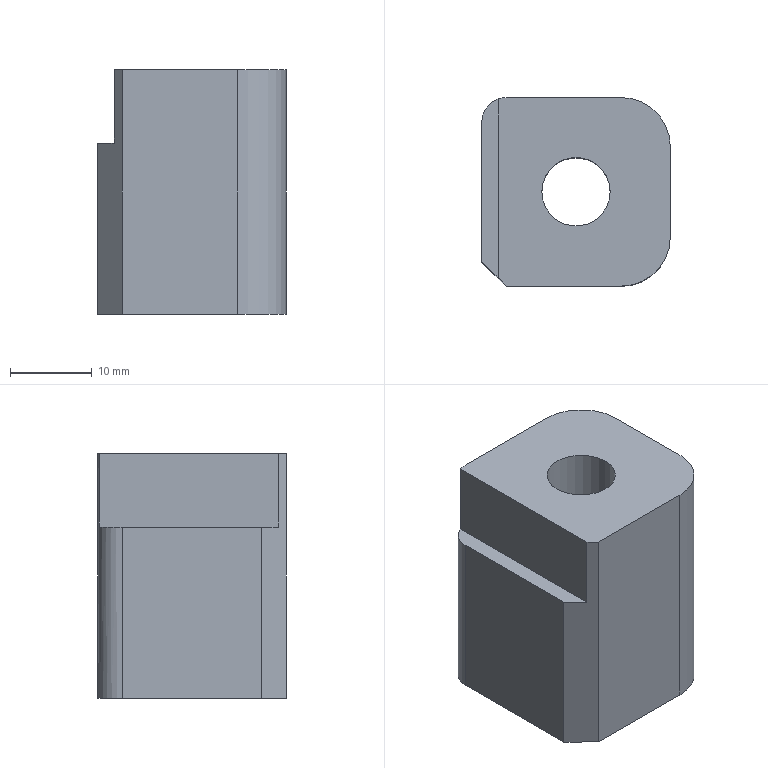Part | STEP file | 1 solid | 13 faces | box 23.1 x 23.1 x 30 mm | volume 13334 mm3 | plane 9 | cylinder 4 | commonest cylinder face diameters 12 x2 6 x1 8.38 x1
STEP:
#1=CARTESIAN_POINT('',(-203.45,11.55,-32.));
#2=VERTEX_POINT('',#1);
#3=CARTESIAN_POINT('',(-217.55,11.55,-32.));
#4=VERTEX_POINT('',#3);
#5=CARTESIAN_POINT('',(-209.,11.55,-32.));
#6=DIRECTION('',(-1.,0.,0.));
#7=VECTOR('',#6,1.);
#8=LINE('',#5,#7);
#9=EDGE_CURVE('',#2,#4,#8,.T.);
#10=ORIENTED_EDGE('',*,*,#9,.T.);
#11=CARTESIAN_POINT('',(-217.55,11.55,-2.));
#12=VERTEX_POINT('',#11);
#13=CARTESIAN_POINT('',(-217.55,11.55,-30.));
#14=DIRECTION('',(0.,0.,1.));
#15=VECTOR('',#14,1.);
#16=LINE('',#13,#15);
#17=EDGE_CURVE('',#4,#12,#16,.T.);
#18=ORIENTED_EDGE('',*,*,#17,.T.);
#19=CARTESIAN_POINT('',(-203.45,11.55,-2.));
#20=VERTEX_POINT('',#19);
#21=CARTESIAN_POINT('',(-209.,11.55,-2.));
#22=DIRECTION('',(1.,0.,0.));
#23=VECTOR('',#22,1.);
#24=LINE('',#21,#23);
#25=EDGE_CURVE('',#12,#20,#24,.T.);
#26=ORIENTED_EDGE('',*,*,#25,.T.);
#27=CARTESIAN_POINT('',(-203.45,11.55,-30.));
#28=DIRECTION('',(0.,0.,-1.));
#29=VECTOR('',#28,1.);
#30=LINE('',#27,#29);
#31=EDGE_CURVE('',#20,#2,#30,.T.);
#32=ORIENTED_EDGE('',*,*,#31,.T.);
#33=EDGE_LOOP('',(#10,#18,#26,#32));
#34=FACE_OUTER_BOUND('',#33,.T.);
#35=CARTESIAN_POINT('',(-209.,11.55,-30.));
#36=DIRECTION('',(0.,1.,0.));
#37=DIRECTION('',(0.,0.,-1.));
#38=AXIS2_PLACEMENT_3D('',#35,#36,#37);
#39=PLANE('',#38);
#40=ADVANCED_FACE('',(#34),#39,.T.);
#41=CARTESIAN_POINT('',(-197.45,5.55,-2.));
#42=VERTEX_POINT('',#41);
#43=CARTESIAN_POINT('',(-197.45,-5.55,-2.));
#44=VERTEX_POINT('',#43);
#45=CARTESIAN_POINT('',(-197.45,0.,-2.));
#46=DIRECTION('',(0.,-1.,0.));
#47=VECTOR('',#46,1.);
#48=LINE('',#45,#47);
#49=EDGE_CURVE('',#42,#44,#48,.T.);
#50=ORIENTED_EDGE('',*,*,#49,.T.);
#51=CARTESIAN_POINT('',(-197.45,-5.55,-32.));
#52=VERTEX_POINT('',#51);
#53=CARTESIAN_POINT('',(-197.45,-5.55,-30.));
#54=DIRECTION('',(0.,0.,-1.));
#55=VECTOR('',#54,1.);
#56=LINE('',#53,#55);
#57=EDGE_CURVE('',#44,#52,#56,.T.);
#58=ORIENTED_EDGE('',*,*,#57,.T.);
#59=CARTESIAN_POINT('',(-197.45,5.55,-32.));
#60=VERTEX_POINT('',#59);
#61=CARTESIAN_POINT('',(-197.45,0.,-32.));
#62=DIRECTION('',(0.,1.,0.));
#63=VECTOR('',#62,1.);
#64=LINE('',#61,#63);
#65=EDGE_CURVE('',#52,#60,#64,.T.);
#66=ORIENTED_EDGE('',*,*,#65,.T.);
#67=CARTESIAN_POINT('',(-197.45,5.55,-30.));
#68=DIRECTION('',(0.,0.,1.));
#69=VECTOR('',#68,1.);
#70=LINE('',#67,#69);
#71=EDGE_CURVE('',#60,#42,#70,.T.);
#72=ORIENTED_EDGE('',*,*,#71,.T.);
#73=EDGE_LOOP('',(#50,#58,#66,#72));
#74=FACE_OUTER_BOUND('',#73,.T.);
#75=CARTESIAN_POINT('',(-197.45,0.,-30.));
#76=DIRECTION('',(1.,0.,0.));
#77=DIRECTION('',(0.,0.,1.));
#78=AXIS2_PLACEMENT_3D('',#75,#76,#77);
#79=PLANE('',#78);
#80=ADVANCED_FACE('',(#74),#79,.T.);
#81=CARTESIAN_POINT('',(-203.45,-11.55,-2.));
#82=VERTEX_POINT('',#81);
#83=CARTESIAN_POINT('',(-217.55,-11.55,-2.));
#84=VERTEX_POINT('',#83);
#85=CARTESIAN_POINT('',(-209.,-11.55,-2.));
#86=DIRECTION('',(-1.,0.,0.));
#87=VECTOR('',#86,1.);
#88=LINE('',#85,#87);
#89=EDGE_CURVE('',#82,#84,#88,.T.);
#90=ORIENTED_EDGE('',*,*,#89,.T.);
#91=CARTESIAN_POINT('',(-217.55,-11.55,-32.));
#92=VERTEX_POINT('',#91);
#93=CARTESIAN_POINT('',(-217.55,-11.55,-30.));
#94=DIRECTION('',(0.,0.,-1.));
#95=VECTOR('',#94,1.);
#96=LINE('',#93,#95);
#97=EDGE_CURVE('',#84,#92,#96,.T.);
#98=ORIENTED_EDGE('',*,*,#97,.T.);
#99=CARTESIAN_POINT('',(-203.45,-11.55,-32.));
#100=VERTEX_POINT('',#99);
#101=CARTESIAN_POINT('',(-209.,-11.55,-32.));
#102=DIRECTION('',(1.,0.,0.));
#103=VECTOR('',#102,1.);
#104=LINE('',#101,#103);
#105=EDGE_CURVE('',#92,#100,#104,.T.);
#106=ORIENTED_EDGE('',*,*,#105,.T.);
#107=CARTESIAN_POINT('',(-203.45,-11.55,-30.));
#108=DIRECTION('',(0.,0.,1.));
#109=VECTOR('',#108,1.);
#110=LINE('',#107,#109);
#111=EDGE_CURVE('',#100,#82,#110,.T.);
#112=ORIENTED_EDGE('',*,*,#111,.T.);
#113=EDGE_LOOP('',(#90,#98,#106,#112));
#114=FACE_OUTER_BOUND('',#113,.T.);
#115=CARTESIAN_POINT('',(-209.,-11.55,-30.));
#116=DIRECTION('',(0.,-1.,0.));
#117=DIRECTION('',(0.,0.,1.));
#118=AXIS2_PLACEMENT_3D('',#115,#116,#117);
#119=PLANE('',#118);
#120=ADVANCED_FACE('',(#114),#119,.T.);
#121=CARTESIAN_POINT('',(-213.19,0.,-32.));
#122=VERTEX_POINT('',#121);
#123=CARTESIAN_POINT('',(-209.,0.,-32.));
#124=DIRECTION('',(0.,0.,1.));
#125=DIRECTION('',(-1.,0.,0.));
#126=AXIS2_PLACEMENT_3D('',#123,#124,#125);
#127=CIRCLE('',#126,4.19);
#128=EDGE_CURVE('',#122,#122,#127,.T.);
#129=ORIENTED_EDGE('',*,*,#128,.T.);
#130=EDGE_LOOP('',(#129));
#131=FACE_BOUND('',#130,.T.);
#132=ORIENTED_EDGE('',*,*,#105,.F.);
#133=CARTESIAN_POINT('',(-220.55,-8.55,-32.));
#134=VERTEX_POINT('',#133);
#135=CARTESIAN_POINT('',(-219.05,-10.05,-32.));
#136=DIRECTION('',(-0.7071,0.7071,0.));
#137=VECTOR('',#136,1.);
#138=LINE('',#135,#137);
#139=EDGE_CURVE('',#92,#134,#138,.T.);
#140=ORIENTED_EDGE('',*,*,#139,.T.);
#141=CARTESIAN_POINT('',(-220.55,8.55,-32.));
#142=VERTEX_POINT('',#141);
#143=CARTESIAN_POINT('',(-220.55,0.,-32.));
#144=DIRECTION('',(0.,-1.,0.));
#145=VECTOR('',#144,1.);
#146=LINE('',#143,#145);
#147=EDGE_CURVE('',#142,#134,#146,.T.);
#148=ORIENTED_EDGE('',*,*,#147,.F.);
#149=CARTESIAN_POINT('',(-217.55,8.55,-32.));
#150=DIRECTION('',(0.,0.,-1.));
#151=DIRECTION('',(-1.,0.,0.));
#152=AXIS2_PLACEMENT_3D('',#149,#150,#151);
#153=CIRCLE('',#152,3.);
#154=EDGE_CURVE('',#142,#4,#153,.T.);
#155=ORIENTED_EDGE('',*,*,#154,.T.);
#156=ORIENTED_EDGE('',*,*,#9,.F.);
#157=CARTESIAN_POINT('',(-203.45,5.55,-32.));
#158=DIRECTION('',(0.,0.,-1.));
#159=DIRECTION('',(-1.,0.,0.));
#160=AXIS2_PLACEMENT_3D('',#157,#158,#159);
#161=CIRCLE('',#160,6.);
#162=EDGE_CURVE('',#2,#60,#161,.T.);
#163=ORIENTED_EDGE('',*,*,#162,.T.);
#164=ORIENTED_EDGE('',*,*,#65,.F.);
#165=CARTESIAN_POINT('',(-203.45,-5.55,-32.));
#166=DIRECTION('',(0.,0.,-1.));
#167=DIRECTION('',(-1.,0.,0.));
#168=AXIS2_PLACEMENT_3D('',#165,#166,#167);
#169=CIRCLE('',#168,6.);
#170=EDGE_CURVE('',#52,#100,#169,.T.);
#171=ORIENTED_EDGE('',*,*,#170,.T.);
#172=EDGE_LOOP('',(#132,#140,#148,#155,#156,#163,#164,#171));
#173=FACE_BOUND('',#172,.T.);
#174=CARTESIAN_POINT('',(-209.,0.,-32.));
#175=DIRECTION('',(0.,0.,-1.));
#176=DIRECTION('',(1.,0.,0.));
#177=AXIS2_PLACEMENT_3D('',#174,#175,#176);
#178=PLANE('',#177);
#179=ADVANCED_FACE('',(#131,#173),#178,.T.);
#180=ORIENTED_EDGE('',*,*,#147,.T.);
#181=CARTESIAN_POINT('',(-220.55,-8.55,-11.));
#182=VERTEX_POINT('',#181);
#183=CARTESIAN_POINT('',(-220.55,-8.55,-30.));
#184=DIRECTION('',(0.,0.,1.));
#185=VECTOR('',#184,1.);
#186=LINE('',#183,#185);
#187=EDGE_CURVE('',#134,#182,#186,.T.);
#188=ORIENTED_EDGE('',*,*,#187,.T.);
#189=CARTESIAN_POINT('',(-220.55,8.55,-11.));
#190=VERTEX_POINT('',#189);
#191=CARTESIAN_POINT('',(-220.55,0.,-11.));
#192=DIRECTION('',(0.,1.,0.));
#193=VECTOR('',#192,1.);
#194=LINE('',#191,#193);
#195=EDGE_CURVE('',#182,#190,#194,.T.);
#196=ORIENTED_EDGE('',*,*,#195,.T.);
#197=CARTESIAN_POINT('',(-220.55,8.55,-30.));
#198=DIRECTION('',(0.,0.,-1.));
#199=VECTOR('',#198,1.);
#200=LINE('',#197,#199);
#201=EDGE_CURVE('',#190,#142,#200,.T.);
#202=ORIENTED_EDGE('',*,*,#201,.T.);
#203=EDGE_LOOP('',(#180,#188,#196,#202));
#204=FACE_OUTER_BOUND('',#203,.T.);
#205=CARTESIAN_POINT('',(-220.55,0.,-30.));
#206=DIRECTION('',(-1.,0.,0.));
#207=DIRECTION('',(0.,0.,-1.));
#208=AXIS2_PLACEMENT_3D('',#205,#206,#207);
#209=PLANE('',#208);
#210=ADVANCED_FACE('',(#204),#209,.T.);
#211=ORIENTED_EDGE('',*,*,#128,.F.);
#212=EDGE_LOOP('',(#211));
#213=FACE_BOUND('',#212,.T.);
#214=CARTESIAN_POINT('',(-204.81,0.,-2.));
#215=VERTEX_POINT('',#214);
#216=CARTESIAN_POINT('',(-209.,0.,-2.));
#217=DIRECTION('',(0.,0.,1.));
#218=DIRECTION('',(1.,0.,0.));
#219=AXIS2_PLACEMENT_3D('',#216,#217,#218);
#220=CIRCLE('',#219,4.19);
#221=EDGE_CURVE('',#215,#215,#220,.T.);
#222=ORIENTED_EDGE('',*,*,#221,.T.);
#223=EDGE_LOOP('',(#222));
#224=FACE_BOUND('',#223,.T.);
#225=CARTESIAN_POINT('',(-209.,0.,-30.));
#226=DIRECTION('',(0.,0.,1.));
#227=DIRECTION('',(1.,0.,0.));
#228=AXIS2_PLACEMENT_3D('',#225,#226,#227);
#229=CYLINDRICAL_SURFACE('',#228,4.19);
#230=ADVANCED_FACE('',(#213,#224),#229,.F.);
#231=ORIENTED_EDGE('',*,*,#195,.F.);
#232=CARTESIAN_POINT('',(-218.55,-10.55,-11.));
#233=VERTEX_POINT('',#232);
#234=CARTESIAN_POINT('',(-220.55,-8.55,-11.));
#235=DIRECTION('',(0.7071,-0.7071,0.));
#236=VECTOR('',#235,1.);
#237=LINE('',#234,#236);
#238=EDGE_CURVE('',#182,#233,#237,.T.);
#239=ORIENTED_EDGE('',*,*,#238,.T.);
#240=CARTESIAN_POINT('',(-218.55,11.378,-11.));
#241=VERTEX_POINT('',#240);
#242=CARTESIAN_POINT('',(-218.55,-1.5,-11.));
#243=DIRECTION('',(0.,1.,0.));
#244=VECTOR('',#243,1.);
#245=LINE('',#242,#244);
#246=EDGE_CURVE('',#233,#241,#245,.T.);
#247=ORIENTED_EDGE('',*,*,#246,.T.);
#248=CARTESIAN_POINT('',(-217.55,8.55,-11.));
#249=DIRECTION('',(0.,0.,1.));
#250=DIRECTION('',(-1.,0.,0.));
#251=AXIS2_PLACEMENT_3D('',#248,#249,#250);
#252=CIRCLE('',#251,3.);
#253=EDGE_CURVE('',#241,#190,#252,.T.);
#254=ORIENTED_EDGE('',*,*,#253,.T.);
#255=EDGE_LOOP('',(#231,#239,#247,#254));
#256=FACE_OUTER_BOUND('',#255,.T.);
#257=CARTESIAN_POINT('',(-209.,0.,-11.));
#258=DIRECTION('',(0.,0.,-1.));
#259=DIRECTION('',(1.,0.,0.));
#260=AXIS2_PLACEMENT_3D('',#257,#258,#259);
#261=PLANE('',#260);
#262=ADVANCED_FACE('',(#256),#261,.F.);
#263=CARTESIAN_POINT('',(-218.55,11.378,-2.));
#264=VERTEX_POINT('',#263);
#265=CARTESIAN_POINT('',(-218.55,-10.55,-2.));
#266=VERTEX_POINT('',#265);
#267=CARTESIAN_POINT('',(-218.55,-1.5,-2.));
#268=DIRECTION('',(0.,-1.,0.));
#269=VECTOR('',#268,1.);
#270=LINE('',#267,#269);
#271=EDGE_CURVE('',#264,#266,#270,.T.);
#272=ORIENTED_EDGE('',*,*,#271,.T.);
#273=CARTESIAN_POINT('',(-219.05,-10.05,-2.));
#274=DIRECTION('',(0.7071,-0.7071,0.));
#275=VECTOR('',#274,1.);
#276=LINE('',#273,#275);
#277=EDGE_CURVE('',#266,#84,#276,.T.);
#278=ORIENTED_EDGE('',*,*,#277,.T.);
#279=ORIENTED_EDGE('',*,*,#89,.F.);
#280=CARTESIAN_POINT('',(-203.45,-5.55,-2.));
#281=DIRECTION('',(0.,0.,1.));
#282=DIRECTION('',(1.,0.,0.));
#283=AXIS2_PLACEMENT_3D('',#280,#281,#282);
#284=CIRCLE('',#283,6.);
#285=EDGE_CURVE('',#82,#44,#284,.T.);
#286=ORIENTED_EDGE('',*,*,#285,.T.);
#287=ORIENTED_EDGE('',*,*,#49,.F.);
#288=CARTESIAN_POINT('',(-203.45,5.55,-2.));
#289=DIRECTION('',(0.,0.,1.));
#290=DIRECTION('',(1.,0.,0.));
#291=AXIS2_PLACEMENT_3D('',#288,#289,#290);
#292=CIRCLE('',#291,6.);
#293=EDGE_CURVE('',#42,#20,#292,.T.);
#294=ORIENTED_EDGE('',*,*,#293,.T.);
#295=ORIENTED_EDGE('',*,*,#25,.F.);
#296=CARTESIAN_POINT('',(-217.55,8.55,-2.));
#297=DIRECTION('',(0.,0.,1.));
#298=DIRECTION('',(1.,0.,0.));
#299=AXIS2_PLACEMENT_3D('',#296,#297,#298);
#300=CIRCLE('',#299,3.);
#301=EDGE_CURVE('',#12,#264,#300,.T.);
#302=ORIENTED_EDGE('',*,*,#301,.T.);
#303=EDGE_LOOP('',(#272,#278,#279,#286,#287,#294,#295,#302));
#304=FACE_BOUND('',#303,.T.);
#305=ORIENTED_EDGE('',*,*,#221,.F.);
#306=EDGE_LOOP('',(#305));
#307=FACE_BOUND('',#306,.T.);
#308=CARTESIAN_POINT('',(-209.,0.,-2.));
#309=DIRECTION('',(0.,0.,1.));
#310=DIRECTION('',(-1.,0.,0.));
#311=AXIS2_PLACEMENT_3D('',#308,#309,#310);
#312=PLANE('',#311);
#313=ADVANCED_FACE('',(#304,#307),#312,.T.);
#314=ORIENTED_EDGE('',*,*,#246,.F.);
#315=CARTESIAN_POINT('',(-218.55,-10.55,-30.));
#316=DIRECTION('',(0.,0.,1.));
#317=VECTOR('',#316,1.);
#318=LINE('',#315,#317);
#319=EDGE_CURVE('',#233,#266,#318,.T.);
#320=ORIENTED_EDGE('',*,*,#319,.T.);
#321=ORIENTED_EDGE('',*,*,#271,.F.);
#322=CARTESIAN_POINT('',(-218.55,11.378,-2.));
#323=DIRECTION('',(0.,0.,-1.));
#324=VECTOR('',#323,1.);
#325=LINE('',#322,#324);
#326=EDGE_CURVE('',#264,#241,#325,.T.);
#327=ORIENTED_EDGE('',*,*,#326,.T.);
#328=EDGE_LOOP('',(#314,#320,#321,#327));
#329=FACE_OUTER_BOUND('',#328,.T.);
#330=CARTESIAN_POINT('',(-218.55,-1.5,-4.5));
#331=DIRECTION('',(1.,0.,0.));
#332=DIRECTION('',(0.,0.,1.));
#333=AXIS2_PLACEMENT_3D('',#330,#331,#332);
#334=PLANE('',#333);
#335=ADVANCED_FACE('',(#329),#334,.F.);
#336=ORIENTED_EDGE('',*,*,#170,.F.);
#337=ORIENTED_EDGE('',*,*,#57,.F.);
#338=ORIENTED_EDGE('',*,*,#285,.F.);
#339=ORIENTED_EDGE('',*,*,#111,.F.);
#340=EDGE_LOOP('',(#336,#337,#338,#339));
#341=FACE_OUTER_BOUND('',#340,.T.);
#342=CARTESIAN_POINT('',(-203.45,-5.55,-30.));
#343=DIRECTION('',(0.,0.,1.));
#344=DIRECTION('',(1.,0.,0.));
#345=AXIS2_PLACEMENT_3D('',#342,#343,#344);
#346=CYLINDRICAL_SURFACE('',#345,6.);
#347=ADVANCED_FACE('',(#341),#346,.T.);
#348=ORIENTED_EDGE('',*,*,#162,.F.);
#349=ORIENTED_EDGE('',*,*,#31,.F.);
#350=ORIENTED_EDGE('',*,*,#293,.F.);
#351=ORIENTED_EDGE('',*,*,#71,.F.);
#352=EDGE_LOOP('',(#348,#349,#350,#351));
#353=FACE_OUTER_BOUND('',#352,.T.);
#354=CARTESIAN_POINT('',(-203.45,5.55,-30.));
#355=DIRECTION('',(0.,0.,1.));
#356=DIRECTION('',(1.,0.,0.));
#357=AXIS2_PLACEMENT_3D('',#354,#355,#356);
#358=CYLINDRICAL_SURFACE('',#357,6.);
#359=ADVANCED_FACE('',(#353),#358,.T.);
#360=ORIENTED_EDGE('',*,*,#301,.F.);
#361=ORIENTED_EDGE('',*,*,#17,.F.);
#362=ORIENTED_EDGE('',*,*,#154,.F.);
#363=ORIENTED_EDGE('',*,*,#201,.F.);
#364=ORIENTED_EDGE('',*,*,#253,.F.);
#365=ORIENTED_EDGE('',*,*,#326,.F.);
#366=EDGE_LOOP('',(#360,#361,#362,#363,#364,#365));
#367=FACE_OUTER_BOUND('',#366,.T.);
#368=CARTESIAN_POINT('',(-217.55,8.55,-30.));
#369=DIRECTION('',(0.,0.,-1.));
#370=DIRECTION('',(-1.,0.,0.));
#371=AXIS2_PLACEMENT_3D('',#368,#369,#370);
#372=CYLINDRICAL_SURFACE('',#371,3.);
#373=ADVANCED_FACE('',(#367),#372,.T.);
#374=ORIENTED_EDGE('',*,*,#139,.F.);
#375=ORIENTED_EDGE('',*,*,#97,.F.);
#376=ORIENTED_EDGE('',*,*,#277,.F.);
#377=ORIENTED_EDGE('',*,*,#319,.F.);
#378=ORIENTED_EDGE('',*,*,#238,.F.);
#379=ORIENTED_EDGE('',*,*,#187,.F.);
#380=EDGE_LOOP('',(#374,#375,#376,#377,#378,#379));
#381=FACE_OUTER_BOUND('',#380,.T.);
#382=CARTESIAN_POINT('',(-220.55,-8.55,-30.));
#383=DIRECTION('',(0.7071,0.7071,0.));
#384=DIRECTION('',(0.,0.,1.));
#385=AXIS2_PLACEMENT_3D('',#382,#383,#384);
#386=PLANE('',#385);
#387=ADVANCED_FACE('',(#381),#386,.F.);
#388=CLOSED_SHELL('',(#40,#80,#120,#179,#210,#230,#262,#313,#335,#347,#359,#373,#387));
#389=MANIFOLD_SOLID_BREP('',#388);
#390=(LENGTH_UNIT()NAMED_UNIT(*)SI_UNIT(.MILLI.,.METRE.));
#391=UNCERTAINTY_MEASURE_WITH_UNIT(LENGTH_MEASURE(0.00002),#390,'','');
#392=(NAMED_UNIT(*)PLANE_ANGLE_UNIT()SI_UNIT($,.RADIAN.));
#393=PLANE_ANGLE_MEASURE_WITH_UNIT(PLANE_ANGLE_MEASURE(0.01745),#392);
#394=DIMENSIONAL_EXPONENTS(0.,0.,0.,0.,0.,0.,0.);
#395=(CONVERSION_BASED_UNIT('DEGREE',#393)NAMED_UNIT(#394)PLANE_ANGLE_UNIT());
#396=(NAMED_UNIT(*)SI_UNIT($,.STERADIAN.)SOLID_ANGLE_UNIT());
#397=(GEOMETRIC_REPRESENTATION_CONTEXT(3)GLOBAL_UNCERTAINTY_ASSIGNED_CONTEXT((#391))GLOBAL_UNIT_ASSIGNED_CONTEXT((#390,#395,#396))REPRESENTATION_CONTEXT('',''));
#398=ADVANCED_BREP_SHAPE_REPRESENTATION('',(#389),#397);